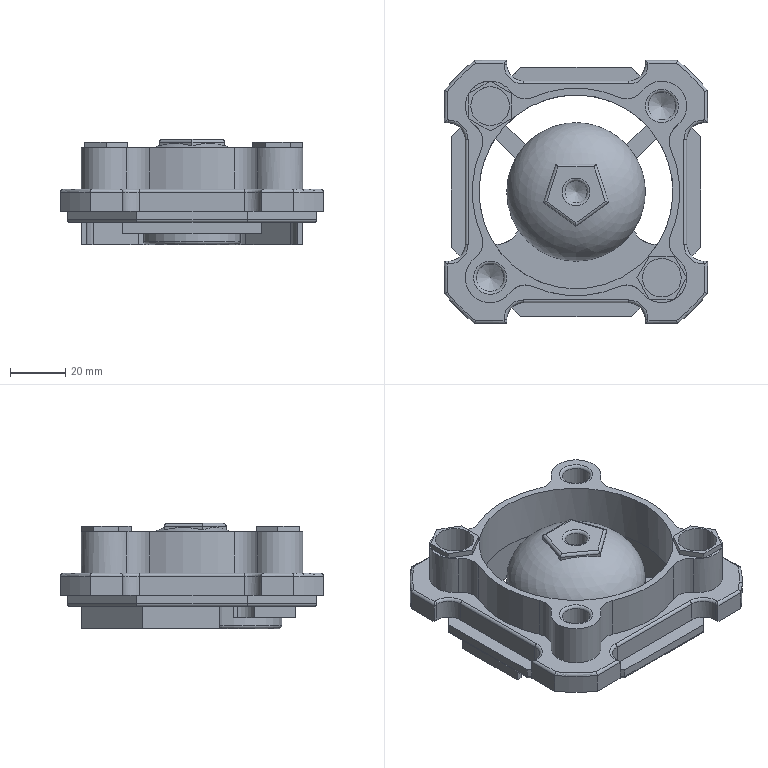CAM job | NX | 3-axis milling, drilling | part box 95 x 95 x 38 mm | stock box 95 x 95 x 38 mm
Tools:
number,name,description,diameter,corner_radius,flute_length,length,flutes
0,D20,Milling Tool-5 Parameters,20.0,0.0,50.0,75.0,2
0,点钻,Drilling Tool,10.0,0.0,35.0,50.0,2
0,D10,Drilling Tool,10.0,0.0,35.0,50.0,2
0,D8,Milling Tool-5 Parameters,8.0,0.0,50.0,75.0,2
0,F10,Milling Tool-5 Parameters,10.0,0.0,50.0,75.0,2
0,D4,Milling Tool-5 Parameters,4.0,0.0,50.0,75.0,2
0,D10R1,Milling Tool-5 Parameters,10.0,1.0,50.0,75.0,2
Operations:
program,operation,operation_type,tool,method,geometry_group,spindle_rpm,surface_speed,feed_per_tooth,feed_cut,feed_plunge,cut_length_mm,path_length_mm,cut_time_min,machine_time_min
PROGRAM,FACE_MILLING,FaceMilling,D20,METHOD,WORKPIECE,3000.0,282.0,0.4167,2500.0,100.0,1013.856,1033.456,0.4055,0.4075
PROGRAM,CAVITY_MILL_COPY,CavityMilling,D20,METHOD,WORKPIECE,3000.0,282.0,0.4167,2500.0,100.0,7496.589,7655.298,2.999,3.014
PROGRAM,CAVITY_MILL,CavityMilling,F10,METHOD,WORKPIECE,3000.0,282.0,0.4167,2500.0,100.0,12802.61,14994.626,5.121,5.34
PROGRAM,PLANAR_MILL,PlanarMilling,D20,METHOD,WORKPIECE,3000.0,282.0,0.4167,2500.0,100.0,8008.717,8266.573,3.204,3.229
PROGRAM,PLANAR_MILL_COPY,PlanarMilling,D20,METHOD,WORKPIECE,3000.0,282.0,0.4167,2500.0,100.0,4848.329,5020.969,1.939,1.957
PROGRAM,SPOT_DRILLING,Operation,点钻,METHOD,WORKPIECE,0.0,0.0,0.0,250.0,0.0,15.0,276.031,0.06,0.0861
PROGRAM,DRILLING,Operation,D10,METHOD,WORKPIECE,0.0,0.0,0.0,250.0,0.0,80.009,408.283,0.32,0.3529
PROGRAM,HOLE_MILLING,CylinderMilling,D8,METHOD,WORKPIECE,3000.0,282.0,0.4167,2500.0,100.0,3261.153,3426.835,1.304,1.321
PROGRAM,FIXED_CONTOUR,SurfaceContour,D4,METHOD,WORKPIECE,3000.0,282.0,0.4167,2500.0,100.0,1377,1390.6,0.5508,0.5522
PROGRAM,FIXED_CONTOUR_1,SurfaceContour,D4,METHOD,WORKPIECE,3000.0,282.0,0.4167,2500.0,100.0,97.646,110.446,0.0391,0.0403
PROGRAM,FIXED_CONTOUR_2,SurfaceContour,D10R1,METHOD,MCS_MILL,3000.0,282.0,0.4167,2500.0,100.0,29291.784,29315.784,11.717,11.719